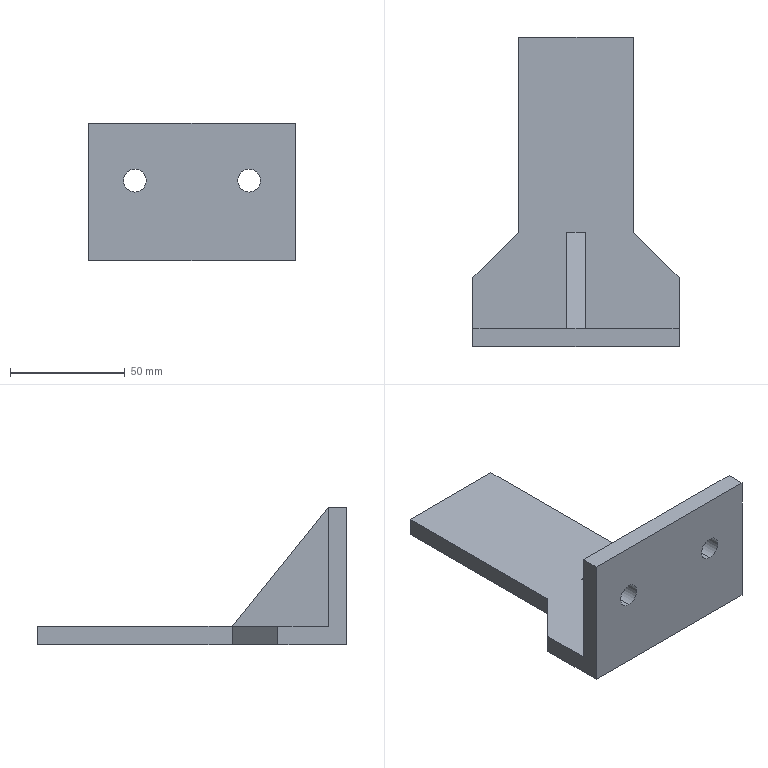Part | SolidWorks | features ICE 6, Extrusion 1 | 1 solid | 20 faces | box 90 x 135 x 60 mm | volume 111719 mm3 | plane 16 | cylinder 4 | commonest cylinder face diameters 10 x4
STEP:
#1=CARTESIAN_POINT('',(70.,0.,30.));
#2=VERTEX_POINT('',#1);
#3=CARTESIAN_POINT('',(70.,0.,40.));
#4=VERTEX_POINT('',#3);
#5=CARTESIAN_POINT('',(70.,0.,35.));
#6=DIRECTION('',(0.,1.,0.));
#7=DIRECTION('',(0.,0.,1.));
#8=AXIS2_PLACEMENT_3D('',#5,#6,#7);
#9=CIRCLE('',#8,5.);
#10=EDGE_CURVE('',#2,#4,#9,.T.);
#11=ORIENTED_EDGE('',*,*,#10,.F.);
#12=CARTESIAN_POINT('',(70.,8.,30.));
#13=VERTEX_POINT('',#12);
#14=CARTESIAN_POINT('',(70.,-2.,30.));
#15=DIRECTION('',(0.,1.,0.));
#16=VECTOR('',#15,1000.);
#17=LINE('',#14,#16);
#18=EDGE_CURVE('',#2,#13,#17,.T.);
#19=ORIENTED_EDGE('',*,*,#18,.T.);
#20=CARTESIAN_POINT('',(70.,8.,40.));
#21=VERTEX_POINT('',#20);
#22=CARTESIAN_POINT('',(70.,8.,35.));
#23=DIRECTION('',(0.,1.,0.));
#24=DIRECTION('',(0.,0.,1.));
#25=AXIS2_PLACEMENT_3D('',#22,#23,#24);
#26=CIRCLE('',#25,5.);
#27=EDGE_CURVE('',#13,#21,#26,.T.);
#28=ORIENTED_EDGE('',*,*,#27,.T.);
#29=CARTESIAN_POINT('',(70.,-2.,40.));
#30=DIRECTION('',(0.,1.,0.));
#31=VECTOR('',#30,1000.);
#32=LINE('',#29,#31);
#33=EDGE_CURVE('',#4,#21,#32,.T.);
#34=ORIENTED_EDGE('',*,*,#33,.F.);
#35=EDGE_LOOP('',(#11,#19,#28,#34));
#36=FACE_OUTER_BOUND('',#35,.T.);
#37=CARTESIAN_POINT('',(70.,-2.,35.));
#38=DIRECTION('',(0.,1.,0.));
#39=DIRECTION('',(0.,0.,1.));
#40=AXIS2_PLACEMENT_3D('',#37,#38,#39);
#41=CYLINDRICAL_SURFACE('',#40,5.);
#42=ADVANCED_FACE('',(#36),#41,.F.);
#43=CARTESIAN_POINT('',(20.,0.,30.));
#44=VERTEX_POINT('',#43);
#45=CARTESIAN_POINT('',(20.,0.,40.));
#46=VERTEX_POINT('',#45);
#47=CARTESIAN_POINT('',(20.,0.,35.));
#48=DIRECTION('',(0.,1.,0.));
#49=DIRECTION('',(0.,0.,1.));
#50=AXIS2_PLACEMENT_3D('',#47,#48,#49);
#51=CIRCLE('',#50,5.);
#52=EDGE_CURVE('',#44,#46,#51,.T.);
#53=ORIENTED_EDGE('',*,*,#52,.F.);
#54=CARTESIAN_POINT('',(20.,8.,30.));
#55=VERTEX_POINT('',#54);
#56=CARTESIAN_POINT('',(20.,-2.,30.));
#57=DIRECTION('',(0.,1.,0.));
#58=VECTOR('',#57,1000.);
#59=LINE('',#56,#58);
#60=EDGE_CURVE('',#44,#55,#59,.T.);
#61=ORIENTED_EDGE('',*,*,#60,.T.);
#62=CARTESIAN_POINT('',(20.,8.,40.));
#63=VERTEX_POINT('',#62);
#64=CARTESIAN_POINT('',(20.,8.,35.));
#65=DIRECTION('',(0.,1.,0.));
#66=DIRECTION('',(0.,0.,1.));
#67=AXIS2_PLACEMENT_3D('',#64,#65,#66);
#68=CIRCLE('',#67,5.);
#69=EDGE_CURVE('',#55,#63,#68,.T.);
#70=ORIENTED_EDGE('',*,*,#69,.T.);
#71=CARTESIAN_POINT('',(20.,-2.,40.));
#72=DIRECTION('',(0.,1.,0.));
#73=VECTOR('',#72,1000.);
#74=LINE('',#71,#73);
#75=EDGE_CURVE('',#46,#63,#74,.T.);
#76=ORIENTED_EDGE('',*,*,#75,.F.);
#77=EDGE_LOOP('',(#53,#61,#70,#76));
#78=FACE_OUTER_BOUND('',#77,.T.);
#79=CARTESIAN_POINT('',(20.,-2.,35.));
#80=DIRECTION('',(0.,1.,0.));
#81=DIRECTION('',(0.,0.,1.));
#82=AXIS2_PLACEMENT_3D('',#79,#80,#81);
#83=CYLINDRICAL_SURFACE('',#82,5.);
#84=ADVANCED_FACE('',(#78),#83,.F.);
#85=CARTESIAN_POINT('',(70.,8.,35.));
#86=DIRECTION('',(0.,1.,0.));
#87=DIRECTION('',(0.,0.,1.));
#88=AXIS2_PLACEMENT_3D('',#85,#86,#87);
#89=CIRCLE('',#88,5.);
#90=EDGE_CURVE('',#21,#13,#89,.T.);
#91=ORIENTED_EDGE('',*,*,#90,.F.);
#92=ORIENTED_EDGE('',*,*,#27,.F.);
#93=EDGE_LOOP('',(#91,#92));
#94=FACE_BOUND('',#93,.T.);
#95=CARTESIAN_POINT('',(49.,8.,60.));
#96=VERTEX_POINT('',#95);
#97=CARTESIAN_POINT('',(49.,8.,8.));
#98=VERTEX_POINT('',#97);
#99=CARTESIAN_POINT('',(49.,8.,8.));
#100=DIRECTION('',(0.,0.,-1.));
#101=VECTOR('',#100,1000.);
#102=LINE('',#99,#101);
#103=EDGE_CURVE('',#96,#98,#102,.T.);
#104=ORIENTED_EDGE('',*,*,#103,.F.);
#105=CARTESIAN_POINT('',(90.,8.,60.));
#106=VERTEX_POINT('',#105);
#107=CARTESIAN_POINT('',(0.,8.,60.));
#108=DIRECTION('',(-1.,0.,0.));
#109=VECTOR('',#108,1000.);
#110=LINE('',#107,#109);
#111=EDGE_CURVE('',#106,#96,#110,.T.);
#112=ORIENTED_EDGE('',*,*,#111,.F.);
#113=CARTESIAN_POINT('',(90.,8.,8.));
#114=VERTEX_POINT('',#113);
#115=CARTESIAN_POINT('',(90.,8.,60.));
#116=DIRECTION('',(0.,0.,-1.));
#117=VECTOR('',#116,1000.);
#118=LINE('',#115,#117);
#119=EDGE_CURVE('',#106,#114,#118,.T.);
#120=ORIENTED_EDGE('',*,*,#119,.T.);
#121=CARTESIAN_POINT('',(0.,8.,8.));
#122=DIRECTION('',(-1.,0.,0.));
#123=VECTOR('',#122,1000.);
#124=LINE('',#121,#123);
#125=EDGE_CURVE('',#114,#98,#124,.T.);
#126=ORIENTED_EDGE('',*,*,#125,.T.);
#127=EDGE_LOOP('',(#104,#112,#120,#126));
#128=FACE_OUTER_BOUND('',#127,.T.);
#129=CARTESIAN_POINT('',(0.,8.,60.));
#130=DIRECTION('',(0.,-1.,0.));
#131=DIRECTION('',(0.,0.,-1.));
#132=AXIS2_PLACEMENT_3D('',#129,#130,#131);
#133=PLANE('',#132);
#134=ADVANCED_FACE('',(#94,#128),#133,.F.);
#135=CARTESIAN_POINT('',(0.,30.,0.));
#136=VERTEX_POINT('',#135);
#137=CARTESIAN_POINT('',(0.,0.,0.));
#138=VERTEX_POINT('',#137);
#139=CARTESIAN_POINT('',(0.,0.,0.));
#140=DIRECTION('',(0.,-1.,0.));
#141=VECTOR('',#140,1000.);
#142=LINE('',#139,#141);
#143=EDGE_CURVE('',#136,#138,#142,.T.);
#144=ORIENTED_EDGE('',*,*,#143,.T.);
#145=CARTESIAN_POINT('',(0.,0.,60.));
#146=VERTEX_POINT('',#145);
#147=CARTESIAN_POINT('',(0.,0.,8.));
#148=DIRECTION('',(0.,0.,-1.));
#149=VECTOR('',#148,1000.);
#150=LINE('',#147,#149);
#151=EDGE_CURVE('',#146,#138,#150,.T.);
#152=ORIENTED_EDGE('',*,*,#151,.F.);
#153=CARTESIAN_POINT('',(0.,8.,60.));
#154=VERTEX_POINT('',#153);
#155=CARTESIAN_POINT('',(0.,0.,60.));
#156=DIRECTION('',(0.,-1.,0.));
#157=VECTOR('',#156,1000.);
#158=LINE('',#155,#157);
#159=EDGE_CURVE('',#154,#146,#158,.T.);
#160=ORIENTED_EDGE('',*,*,#159,.F.);
#161=CARTESIAN_POINT('',(0.,8.,8.));
#162=VERTEX_POINT('',#161);
#163=CARTESIAN_POINT('',(0.,8.,60.));
#164=DIRECTION('',(0.,0.,-1.));
#165=VECTOR('',#164,1000.);
#166=LINE('',#163,#165);
#167=EDGE_CURVE('',#154,#162,#166,.T.);
#168=ORIENTED_EDGE('',*,*,#167,.T.);
#169=CARTESIAN_POINT('',(0.,30.,8.));
#170=VERTEX_POINT('',#169);
#171=CARTESIAN_POINT('',(0.,0.,8.));
#172=DIRECTION('',(0.,-1.,0.));
#173=VECTOR('',#172,1000.);
#174=LINE('',#171,#173);
#175=EDGE_CURVE('',#170,#162,#174,.T.);
#176=ORIENTED_EDGE('',*,*,#175,.F.);
#177=CARTESIAN_POINT('',(0.,30.,8.));
#178=DIRECTION('',(0.,0.,-1.));
#179=VECTOR('',#178,1000.);
#180=LINE('',#177,#179);
#181=EDGE_CURVE('',#170,#136,#180,.T.);
#182=ORIENTED_EDGE('',*,*,#181,.T.);
#183=EDGE_LOOP('',(#144,#152,#160,#168,#176,#182));
#184=FACE_OUTER_BOUND('',#183,.T.);
#185=CARTESIAN_POINT('',(0.,0.,8.));
#186=DIRECTION('',(1.,0.,0.));
#187=DIRECTION('',(0.,0.,-1.));
#188=AXIS2_PLACEMENT_3D('',#185,#186,#187);
#189=PLANE('',#188);
#190=ADVANCED_FACE('',(#184),#189,.F.);
#191=CARTESIAN_POINT('',(20.,0.,35.));
#192=DIRECTION('',(0.,1.,0.));
#193=DIRECTION('',(0.,0.,1.));
#194=AXIS2_PLACEMENT_3D('',#191,#192,#193);
#195=CIRCLE('',#194,5.);
#196=EDGE_CURVE('',#46,#44,#195,.T.);
#197=ORIENTED_EDGE('',*,*,#196,.T.);
#198=ORIENTED_EDGE('',*,*,#52,.T.);
#199=EDGE_LOOP('',(#197,#198));
#200=FACE_BOUND('',#199,.T.);
#201=CARTESIAN_POINT('',(70.,0.,35.));
#202=DIRECTION('',(0.,1.,0.));
#203=DIRECTION('',(0.,0.,1.));
#204=AXIS2_PLACEMENT_3D('',#201,#202,#203);
#205=CIRCLE('',#204,5.);
#206=EDGE_CURVE('',#4,#2,#205,.T.);
#207=ORIENTED_EDGE('',*,*,#206,.T.);
#208=ORIENTED_EDGE('',*,*,#10,.T.);
#209=EDGE_LOOP('',(#207,#208));
#210=FACE_BOUND('',#209,.T.);
#211=CARTESIAN_POINT('',(90.,0.,0.));
#212=VERTEX_POINT('',#211);
#213=CARTESIAN_POINT('',(0.,0.,0.));
#214=DIRECTION('',(1.,0.,0.));
#215=VECTOR('',#214,1000.);
#216=LINE('',#213,#215);
#217=EDGE_CURVE('',#138,#212,#216,.T.);
#218=ORIENTED_EDGE('',*,*,#217,.T.);
#219=CARTESIAN_POINT('',(90.,0.,60.));
#220=VERTEX_POINT('',#219);
#221=CARTESIAN_POINT('',(90.,0.,8.));
#222=DIRECTION('',(0.,0.,-1.));
#223=VECTOR('',#222,1000.);
#224=LINE('',#221,#223);
#225=EDGE_CURVE('',#220,#212,#224,.T.);
#226=ORIENTED_EDGE('',*,*,#225,.F.);
#227=CARTESIAN_POINT('',(90.,0.,60.));
#228=DIRECTION('',(1.,0.,0.));
#229=VECTOR('',#228,1000.);
#230=LINE('',#227,#229);
#231=EDGE_CURVE('',#146,#220,#230,.T.);
#232=ORIENTED_EDGE('',*,*,#231,.F.);
#233=ORIENTED_EDGE('',*,*,#151,.T.);
#234=EDGE_LOOP('',(#218,#226,#232,#233));
#235=FACE_OUTER_BOUND('',#234,.T.);
#236=CARTESIAN_POINT('',(0.,0.,8.));
#237=DIRECTION('',(0.,1.,0.));
#238=DIRECTION('',(0.,0.,1.));
#239=AXIS2_PLACEMENT_3D('',#236,#237,#238);
#240=PLANE('',#239);
#241=ADVANCED_FACE('',(#200,#210,#235),#240,.F.);
#242=CARTESIAN_POINT('',(90.,30.,0.));
#243=VERTEX_POINT('',#242);
#244=CARTESIAN_POINT('',(90.,0.,0.));
#245=DIRECTION('',(0.,1.,0.));
#246=VECTOR('',#245,1000.);
#247=LINE('',#244,#246);
#248=EDGE_CURVE('',#212,#243,#247,.T.);
#249=ORIENTED_EDGE('',*,*,#248,.T.);
#250=CARTESIAN_POINT('',(90.,30.,8.));
#251=VERTEX_POINT('',#250);
#252=CARTESIAN_POINT('',(90.,30.,8.));
#253=DIRECTION('',(0.,0.,-1.));
#254=VECTOR('',#253,1000.);
#255=LINE('',#252,#254);
#256=EDGE_CURVE('',#251,#243,#255,.T.);
#257=ORIENTED_EDGE('',*,*,#256,.F.);
#258=CARTESIAN_POINT('',(90.,0.,8.));
#259=DIRECTION('',(0.,1.,0.));
#260=VECTOR('',#259,1000.);
#261=LINE('',#258,#260);
#262=EDGE_CURVE('',#114,#251,#261,.T.);
#263=ORIENTED_EDGE('',*,*,#262,.F.);
#264=ORIENTED_EDGE('',*,*,#119,.F.);
#265=CARTESIAN_POINT('',(90.,8.,60.));
#266=DIRECTION('',(0.,1.,0.));
#267=VECTOR('',#266,1000.);
#268=LINE('',#265,#267);
#269=EDGE_CURVE('',#220,#106,#268,.T.);
#270=ORIENTED_EDGE('',*,*,#269,.F.);
#271=ORIENTED_EDGE('',*,*,#225,.T.);
#272=EDGE_LOOP('',(#249,#257,#263,#264,#270,#271));
#273=FACE_OUTER_BOUND('',#272,.T.);
#274=CARTESIAN_POINT('',(90.,0.,8.));
#275=DIRECTION('',(-1.,0.,0.));
#276=DIRECTION('',(0.,0.,1.));
#277=AXIS2_PLACEMENT_3D('',#274,#275,#276);
#278=PLANE('',#277);
#279=ADVANCED_FACE('',(#273),#278,.F.);
#280=CARTESIAN_POINT('',(70.,50.,0.));
#281=VERTEX_POINT('',#280);
#282=CARTESIAN_POINT('',(70.,50.,0.));
#283=DIRECTION('',(-0.7071,0.7071,0.));
#284=VECTOR('',#283,1000.);
#285=LINE('',#282,#284);
#286=EDGE_CURVE('',#243,#281,#285,.T.);
#287=ORIENTED_EDGE('',*,*,#286,.T.);
#288=CARTESIAN_POINT('',(70.,50.,8.));
#289=VERTEX_POINT('',#288);
#290=CARTESIAN_POINT('',(70.,50.,8.));
#291=DIRECTION('',(0.,0.,-1.));
#292=VECTOR('',#291,1000.);
#293=LINE('',#290,#292);
#294=EDGE_CURVE('',#289,#281,#293,.T.);
#295=ORIENTED_EDGE('',*,*,#294,.F.);
#296=CARTESIAN_POINT('',(70.,50.,8.));
#297=DIRECTION('',(-0.7071,0.7071,0.));
#298=VECTOR('',#297,1000.);
#299=LINE('',#296,#298);
#300=EDGE_CURVE('',#251,#289,#299,.T.);
#301=ORIENTED_EDGE('',*,*,#300,.F.);
#302=ORIENTED_EDGE('',*,*,#256,.T.);
#303=EDGE_LOOP('',(#287,#295,#301,#302));
#304=FACE_OUTER_BOUND('',#303,.T.);
#305=CARTESIAN_POINT('',(70.,50.,8.));
#306=DIRECTION('',(-0.7071,-0.7071,0.));
#307=DIRECTION('',(0.7071,-0.7071,0.));
#308=AXIS2_PLACEMENT_3D('',#305,#306,#307);
#309=PLANE('',#308);
#310=ADVANCED_FACE('',(#304),#309,.F.);
#311=CARTESIAN_POINT('',(70.,135.,0.));
#312=VERTEX_POINT('',#311);
#313=CARTESIAN_POINT('',(70.,135.,0.));
#314=DIRECTION('',(0.,1.,0.));
#315=VECTOR('',#314,1000.);
#316=LINE('',#313,#315);
#317=EDGE_CURVE('',#281,#312,#316,.T.);
#318=ORIENTED_EDGE('',*,*,#317,.T.);
#319=CARTESIAN_POINT('',(70.,135.,8.));
#320=VERTEX_POINT('',#319);
#321=CARTESIAN_POINT('',(70.,135.,8.));
#322=DIRECTION('',(0.,0.,-1.));
#323=VECTOR('',#322,1000.);
#324=LINE('',#321,#323);
#325=EDGE_CURVE('',#320,#312,#324,.T.);
#326=ORIENTED_EDGE('',*,*,#325,.F.);
#327=CARTESIAN_POINT('',(70.,135.,8.));
#328=DIRECTION('',(0.,1.,0.));
#329=VECTOR('',#328,1000.);
#330=LINE('',#327,#329);
#331=EDGE_CURVE('',#289,#320,#330,.T.);
#332=ORIENTED_EDGE('',*,*,#331,.F.);
#333=ORIENTED_EDGE('',*,*,#294,.T.);
#334=EDGE_LOOP('',(#318,#326,#332,#333));
#335=FACE_OUTER_BOUND('',#334,.T.);
#336=CARTESIAN_POINT('',(70.,135.,8.));
#337=DIRECTION('',(-1.,0.,0.));
#338=DIRECTION('',(0.,-1.,0.));
#339=AXIS2_PLACEMENT_3D('',#336,#337,#338);
#340=PLANE('',#339);
#341=ADVANCED_FACE('',(#335),#340,.F.);
#342=CARTESIAN_POINT('',(20.,135.,0.));
#343=VERTEX_POINT('',#342);
#344=CARTESIAN_POINT('',(45.,135.,0.));
#345=DIRECTION('',(-1.,0.,0.));
#346=VECTOR('',#345,1000.);
#347=LINE('',#344,#346);
#348=EDGE_CURVE('',#312,#343,#347,.T.);
#349=ORIENTED_EDGE('',*,*,#348,.T.);
#350=CARTESIAN_POINT('',(20.,135.,8.));
#351=VERTEX_POINT('',#350);
#352=CARTESIAN_POINT('',(20.,135.,8.));
#353=DIRECTION('',(0.,0.,-1.));
#354=VECTOR('',#353,1000.);
#355=LINE('',#352,#354);
#356=EDGE_CURVE('',#351,#343,#355,.T.);
#357=ORIENTED_EDGE('',*,*,#356,.F.);
#358=CARTESIAN_POINT('',(45.,135.,8.));
#359=DIRECTION('',(-1.,0.,0.));
#360=VECTOR('',#359,1000.);
#361=LINE('',#358,#360);
#362=EDGE_CURVE('',#320,#351,#361,.T.);
#363=ORIENTED_EDGE('',*,*,#362,.F.);
#364=ORIENTED_EDGE('',*,*,#325,.T.);
#365=EDGE_LOOP('',(#349,#357,#363,#364));
#366=FACE_OUTER_BOUND('',#365,.T.);
#367=CARTESIAN_POINT('',(45.,135.,8.));
#368=DIRECTION('',(0.,-1.,0.));
#369=DIRECTION('',(0.,0.,-1.));
#370=AXIS2_PLACEMENT_3D('',#367,#368,#369);
#371=PLANE('',#370);
#372=ADVANCED_FACE('',(#366),#371,.F.);
#373=CARTESIAN_POINT('',(20.,50.,0.));
#374=VERTEX_POINT('',#373);
#375=CARTESIAN_POINT('',(20.,135.,0.));
#376=DIRECTION('',(0.,-1.,0.));
#377=VECTOR('',#376,1000.);
#378=LINE('',#375,#377);
#379=EDGE_CURVE('',#343,#374,#378,.T.);
#380=ORIENTED_EDGE('',*,*,#379,.T.);
#381=CARTESIAN_POINT('',(20.,50.,8.));
#382=VERTEX_POINT('',#381);
#383=CARTESIAN_POINT('',(20.,50.,8.));
#384=DIRECTION('',(0.,0.,-1.));
#385=VECTOR('',#384,1000.);
#386=LINE('',#383,#385);
#387=EDGE_CURVE('',#382,#374,#386,.T.);
#388=ORIENTED_EDGE('',*,*,#387,.F.);
#389=CARTESIAN_POINT('',(20.,135.,8.));
#390=DIRECTION('',(0.,-1.,0.));
#391=VECTOR('',#390,1000.);
#392=LINE('',#389,#391);
#393=EDGE_CURVE('',#351,#382,#392,.T.);
#394=ORIENTED_EDGE('',*,*,#393,.F.);
#395=ORIENTED_EDGE('',*,*,#356,.T.);
#396=EDGE_LOOP('',(#380,#388,#394,#395));
#397=FACE_OUTER_BOUND('',#396,.T.);
#398=CARTESIAN_POINT('',(20.,135.,8.));
#399=DIRECTION('',(1.,0.,0.));
#400=DIRECTION('',(0.,1.,0.));
#401=AXIS2_PLACEMENT_3D('',#398,#399,#400);
#402=PLANE('',#401);
#403=ADVANCED_FACE('',(#397),#402,.F.);
#404=CARTESIAN_POINT('',(20.,50.,0.));
#405=DIRECTION('',(-0.7071,-0.7071,0.));
#406=VECTOR('',#405,1000.);
#407=LINE('',#404,#406);
#408=EDGE_CURVE('',#374,#136,#407,.T.);
#409=ORIENTED_EDGE('',*,*,#408,.T.);
#410=ORIENTED_EDGE('',*,*,#181,.F.);
#411=CARTESIAN_POINT('',(20.,50.,8.));
#412=DIRECTION('',(-0.7071,-0.7071,0.));
#413=VECTOR('',#412,1000.);
#414=LINE('',#411,#413);
#415=EDGE_CURVE('',#382,#170,#414,.T.);
#416=ORIENTED_EDGE('',*,*,#415,.F.);
#417=ORIENTED_EDGE('',*,*,#387,.T.);
#418=EDGE_LOOP('',(#409,#410,#416,#417));
#419=FACE_OUTER_BOUND('',#418,.T.);
#420=CARTESIAN_POINT('',(20.,50.,8.));
#421=DIRECTION('',(0.7071,-0.7071,0.));
#422=DIRECTION('',(0.7071,0.7071,0.));
#423=AXIS2_PLACEMENT_3D('',#420,#421,#422);
#424=PLANE('',#423);
#425=ADVANCED_FACE('',(#419),#424,.F.);
#426=CARTESIAN_POINT('',(41.,8.,8.));
#427=VERTEX_POINT('',#426);
#428=CARTESIAN_POINT('',(41.,50.,8.));
#429=VERTEX_POINT('',#428);
#430=CARTESIAN_POINT('',(41.,8.,8.));
#431=DIRECTION('',(0.,1.,0.));
#432=VECTOR('',#431,1000.);
#433=LINE('',#430,#432);
#434=EDGE_CURVE('',#427,#429,#433,.T.);
#435=ORIENTED_EDGE('',*,*,#434,.T.);
#436=CARTESIAN_POINT('',(49.,50.,8.));
#437=VERTEX_POINT('',#436);
#438=CARTESIAN_POINT('',(41.,50.,8.));
#439=DIRECTION('',(1.,0.,0.));
#440=VECTOR('',#439,1000.);
#441=LINE('',#438,#440);
#442=EDGE_CURVE('',#429,#437,#441,.T.);
#443=ORIENTED_EDGE('',*,*,#442,.T.);
#444=CARTESIAN_POINT('',(49.,8.,8.));
#445=DIRECTION('',(0.,1.,0.));
#446=VECTOR('',#445,1000.);
#447=LINE('',#444,#446);
#448=EDGE_CURVE('',#98,#437,#447,.T.);
#449=ORIENTED_EDGE('',*,*,#448,.F.);
#450=ORIENTED_EDGE('',*,*,#125,.F.);
#451=ORIENTED_EDGE('',*,*,#262,.T.);
#452=ORIENTED_EDGE('',*,*,#300,.T.);
#453=ORIENTED_EDGE('',*,*,#331,.T.);
#454=ORIENTED_EDGE('',*,*,#362,.T.);
#455=ORIENTED_EDGE('',*,*,#393,.T.);
#456=ORIENTED_EDGE('',*,*,#415,.T.);
#457=ORIENTED_EDGE('',*,*,#175,.T.);
#458=CARTESIAN_POINT('',(0.,8.,8.));
#459=DIRECTION('',(-1.,0.,0.));
#460=VECTOR('',#459,1000.);
#461=LINE('',#458,#460);
#462=EDGE_CURVE('',#427,#162,#461,.T.);
#463=ORIENTED_EDGE('',*,*,#462,.F.);
#464=EDGE_LOOP('',(#435,#443,#449,#450,#451,#452,#453,#454,#455,#456,#457,#463));
#465=FACE_OUTER_BOUND('',#464,.T.);
#466=CARTESIAN_POINT('',(0.,0.,8.));
#467=DIRECTION('',(0.,0.,1.));
#468=DIRECTION('',(1.,0.,0.));
#469=AXIS2_PLACEMENT_3D('',#466,#467,#468);
#470=PLANE('',#469);
#471=ADVANCED_FACE('',(#465),#470,.T.);
#472=ORIENTED_EDGE('',*,*,#143,.F.);
#473=ORIENTED_EDGE('',*,*,#408,.F.);
#474=ORIENTED_EDGE('',*,*,#379,.F.);
#475=ORIENTED_EDGE('',*,*,#348,.F.);
#476=ORIENTED_EDGE('',*,*,#317,.F.);
#477=ORIENTED_EDGE('',*,*,#286,.F.);
#478=ORIENTED_EDGE('',*,*,#248,.F.);
#479=ORIENTED_EDGE('',*,*,#217,.F.);
#480=EDGE_LOOP('',(#472,#473,#474,#475,#476,#477,#478,#479));
#481=FACE_OUTER_BOUND('',#480,.T.);
#482=CARTESIAN_POINT('',(0.,0.,0.));
#483=DIRECTION('',(0.,0.,1.));
#484=DIRECTION('',(1.,0.,0.));
#485=AXIS2_PLACEMENT_3D('',#482,#483,#484);
#486=PLANE('',#485);
#487=ADVANCED_FACE('',(#481),#486,.F.);
#488=CARTESIAN_POINT('',(20.,8.,35.));
#489=DIRECTION('',(0.,1.,0.));
#490=DIRECTION('',(0.,0.,1.));
#491=AXIS2_PLACEMENT_3D('',#488,#489,#490);
#492=CIRCLE('',#491,5.);
#493=EDGE_CURVE('',#63,#55,#492,.T.);
#494=ORIENTED_EDGE('',*,*,#493,.F.);
#495=ORIENTED_EDGE('',*,*,#69,.F.);
#496=EDGE_LOOP('',(#494,#495));
#497=FACE_BOUND('',#496,.T.);
#498=CARTESIAN_POINT('',(41.,8.,60.));
#499=VERTEX_POINT('',#498);
#500=CARTESIAN_POINT('',(0.,8.,60.));
#501=DIRECTION('',(-1.,0.,0.));
#502=VECTOR('',#501,1000.);
#503=LINE('',#500,#502);
#504=EDGE_CURVE('',#499,#154,#503,.T.);
#505=ORIENTED_EDGE('',*,*,#504,.F.);
#506=CARTESIAN_POINT('',(41.,8.,8.));
#507=DIRECTION('',(0.,0.,-1.));
#508=VECTOR('',#507,1000.);
#509=LINE('',#506,#508);
#510=EDGE_CURVE('',#499,#427,#509,.T.);
#511=ORIENTED_EDGE('',*,*,#510,.T.);
#512=ORIENTED_EDGE('',*,*,#462,.T.);
#513=ORIENTED_EDGE('',*,*,#167,.F.);
#514=EDGE_LOOP('',(#505,#511,#512,#513));
#515=FACE_OUTER_BOUND('',#514,.T.);
#516=CARTESIAN_POINT('',(0.,8.,60.));
#517=DIRECTION('',(0.,-1.,0.));
#518=DIRECTION('',(0.,0.,-1.));
#519=AXIS2_PLACEMENT_3D('',#516,#517,#518);
#520=PLANE('',#519);
#521=ADVANCED_FACE('',(#497,#515),#520,.F.);
#522=ORIENTED_EDGE('',*,*,#231,.T.);
#523=ORIENTED_EDGE('',*,*,#269,.T.);
#524=ORIENTED_EDGE('',*,*,#111,.T.);
#525=CARTESIAN_POINT('',(41.,8.,60.));
#526=DIRECTION('',(1.,0.,0.));
#527=VECTOR('',#526,1000.);
#528=LINE('',#525,#527);
#529=EDGE_CURVE('',#499,#96,#528,.T.);
#530=ORIENTED_EDGE('',*,*,#529,.F.);
#531=ORIENTED_EDGE('',*,*,#504,.T.);
#532=ORIENTED_EDGE('',*,*,#159,.T.);
#533=EDGE_LOOP('',(#522,#523,#524,#530,#531,#532));
#534=FACE_OUTER_BOUND('',#533,.T.);
#535=CARTESIAN_POINT('',(0.,0.,60.));
#536=DIRECTION('',(0.,0.,-1.));
#537=DIRECTION('',(-1.,0.,0.));
#538=AXIS2_PLACEMENT_3D('',#535,#536,#537);
#539=PLANE('',#538);
#540=ADVANCED_FACE('',(#534),#539,.F.);
#541=ORIENTED_EDGE('',*,*,#529,.T.);
#542=CARTESIAN_POINT('',(49.,8.,60.));
#543=DIRECTION('',(0.,-0.6283,0.7779));
#544=VECTOR('',#543,1000.);
#545=LINE('',#542,#544);
#546=EDGE_CURVE('',#437,#96,#545,.T.);
#547=ORIENTED_EDGE('',*,*,#546,.F.);
#548=ORIENTED_EDGE('',*,*,#442,.F.);
#549=CARTESIAN_POINT('',(41.,8.,60.));
#550=DIRECTION('',(0.,-0.6283,0.7779));
#551=VECTOR('',#550,1000.);
#552=LINE('',#549,#551);
#553=EDGE_CURVE('',#429,#499,#552,.T.);
#554=ORIENTED_EDGE('',*,*,#553,.T.);
#555=EDGE_LOOP('',(#541,#547,#548,#554));
#556=FACE_OUTER_BOUND('',#555,.T.);
#557=CARTESIAN_POINT('',(41.,8.,60.));
#558=DIRECTION('',(0.,0.7779,0.6283));
#559=DIRECTION('',(0.,-0.6283,0.7779));
#560=AXIS2_PLACEMENT_3D('',#557,#558,#559);
#561=PLANE('',#560);
#562=ADVANCED_FACE('',(#556),#561,.T.);
#563=ORIENTED_EDGE('',*,*,#510,.F.);
#564=ORIENTED_EDGE('',*,*,#553,.F.);
#565=ORIENTED_EDGE('',*,*,#434,.F.);
#566=EDGE_LOOP('',(#563,#564,#565));
#567=FACE_OUTER_BOUND('',#566,.T.);
#568=CARTESIAN_POINT('',(41.,0.,0.));
#569=DIRECTION('',(-1.,0.,0.));
#570=DIRECTION('',(0.,0.,1.));
#571=AXIS2_PLACEMENT_3D('',#568,#569,#570);
#572=PLANE('',#571);
#573=ADVANCED_FACE('',(#567),#572,.T.);
#574=ORIENTED_EDGE('',*,*,#103,.T.);
#575=ORIENTED_EDGE('',*,*,#448,.T.);
#576=ORIENTED_EDGE('',*,*,#546,.T.);
#577=EDGE_LOOP('',(#574,#575,#576));
#578=FACE_OUTER_BOUND('',#577,.T.);
#579=CARTESIAN_POINT('',(49.,0.,0.));
#580=DIRECTION('',(-1.,0.,0.));
#581=DIRECTION('',(0.,0.,1.));
#582=AXIS2_PLACEMENT_3D('',#579,#580,#581);
#583=PLANE('',#582);
#584=ADVANCED_FACE('',(#578),#583,.F.);
#585=ORIENTED_EDGE('',*,*,#60,.F.);
#586=ORIENTED_EDGE('',*,*,#196,.F.);
#587=ORIENTED_EDGE('',*,*,#75,.T.);
#588=ORIENTED_EDGE('',*,*,#493,.T.);
#589=EDGE_LOOP('',(#585,#586,#587,#588));
#590=FACE_OUTER_BOUND('',#589,.T.);
#591=CARTESIAN_POINT('',(20.,-2.,35.));
#592=DIRECTION('',(0.,1.,0.));
#593=DIRECTION('',(0.,0.,1.));
#594=AXIS2_PLACEMENT_3D('',#591,#592,#593);
#595=CYLINDRICAL_SURFACE('',#594,5.);
#596=ADVANCED_FACE('',(#590),#595,.F.);
#597=ORIENTED_EDGE('',*,*,#18,.F.);
#598=ORIENTED_EDGE('',*,*,#206,.F.);
#599=ORIENTED_EDGE('',*,*,#33,.T.);
#600=ORIENTED_EDGE('',*,*,#90,.T.);
#601=EDGE_LOOP('',(#597,#598,#599,#600));
#602=FACE_OUTER_BOUND('',#601,.T.);
#603=CARTESIAN_POINT('',(70.,-2.,35.));
#604=DIRECTION('',(0.,1.,0.));
#605=DIRECTION('',(0.,0.,1.));
#606=AXIS2_PLACEMENT_3D('',#603,#604,#605);
#607=CYLINDRICAL_SURFACE('',#606,5.);
#608=ADVANCED_FACE('',(#602),#607,.F.);
#609=CLOSED_SHELL('',(#42,#84,#134,#190,#241,#279,#310,#341,#372,#403,#425,#471,#487,#521,#540,#562,#573,#584,#596,#608));
#610=MANIFOLD_SOLID_BREP('',#609);
#611=CARTESIAN_POINT('',(0.,0.,0.));
#612=DIRECTION('',(0.,0.,1.));
#613=DIRECTION('',(1.,0.,0.));
#614=AXIS2_PLACEMENT_3D('',#611,#612,#613);
#615=(LENGTH_UNIT()NAMED_UNIT(*)SI_UNIT(.MILLI.,.METRE.));
#616=UNCERTAINTY_MEASURE_WITH_UNIT(LENGTH_MEASURE(0.00001),#615,'','');
#617=(NAMED_UNIT(*)PLANE_ANGLE_UNIT()SI_UNIT($,.RADIAN.));
#618=(NAMED_UNIT(*)SI_UNIT($,.STERADIAN.)SOLID_ANGLE_UNIT());
#619=(GEOMETRIC_REPRESENTATION_CONTEXT(3)GLOBAL_UNCERTAINTY_ASSIGNED_CONTEXT((#616))GLOBAL_UNIT_ASSIGNED_CONTEXT((#615,#617,#618))REPRESENTATION_CONTEXT('',''));
#620=ADVANCED_BREP_SHAPE_REPRESENTATION('',(#610,#614),#619);